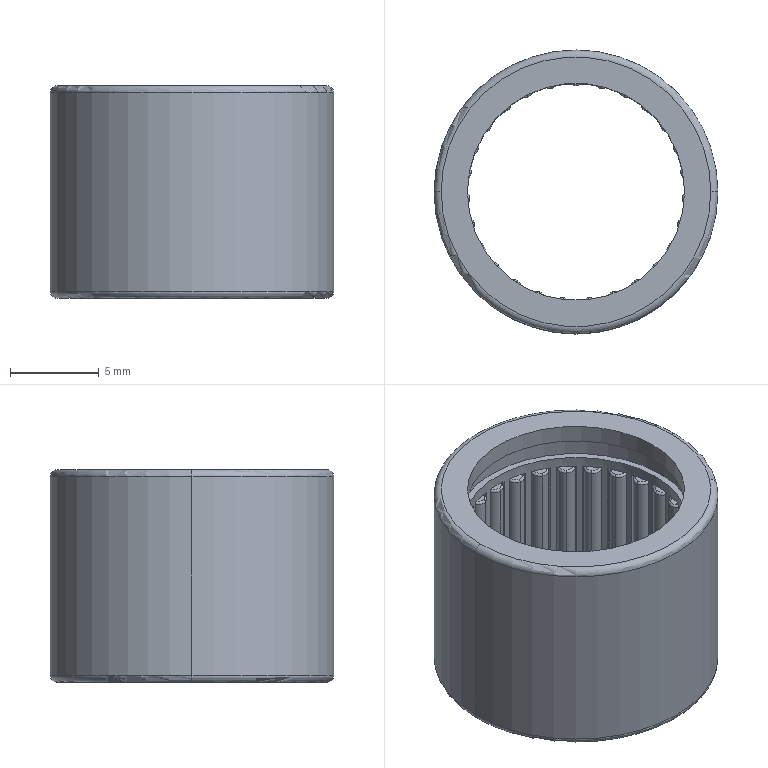Part | SolidWorks | features CirPattern 2, Revolution 2, RevCut 1 | 29 solids | 373 faces | box 16 x 16 x 12 mm | volume 801.274 mm3 | cylinder 147 | plane 114 | torus 112 | commonest cylinder face diameters 1.2 x81 1 x54 12.24 x4 12.62 x2 13.38 x2 14 x2